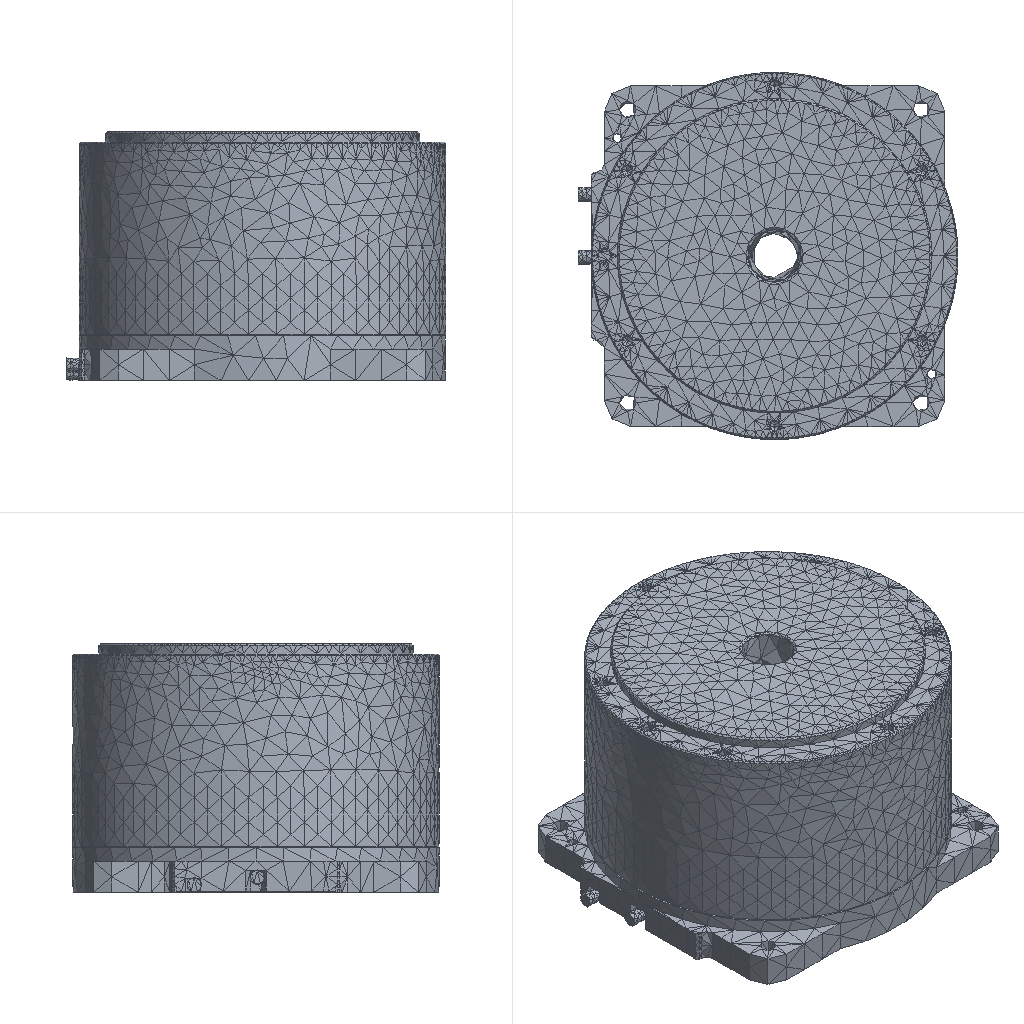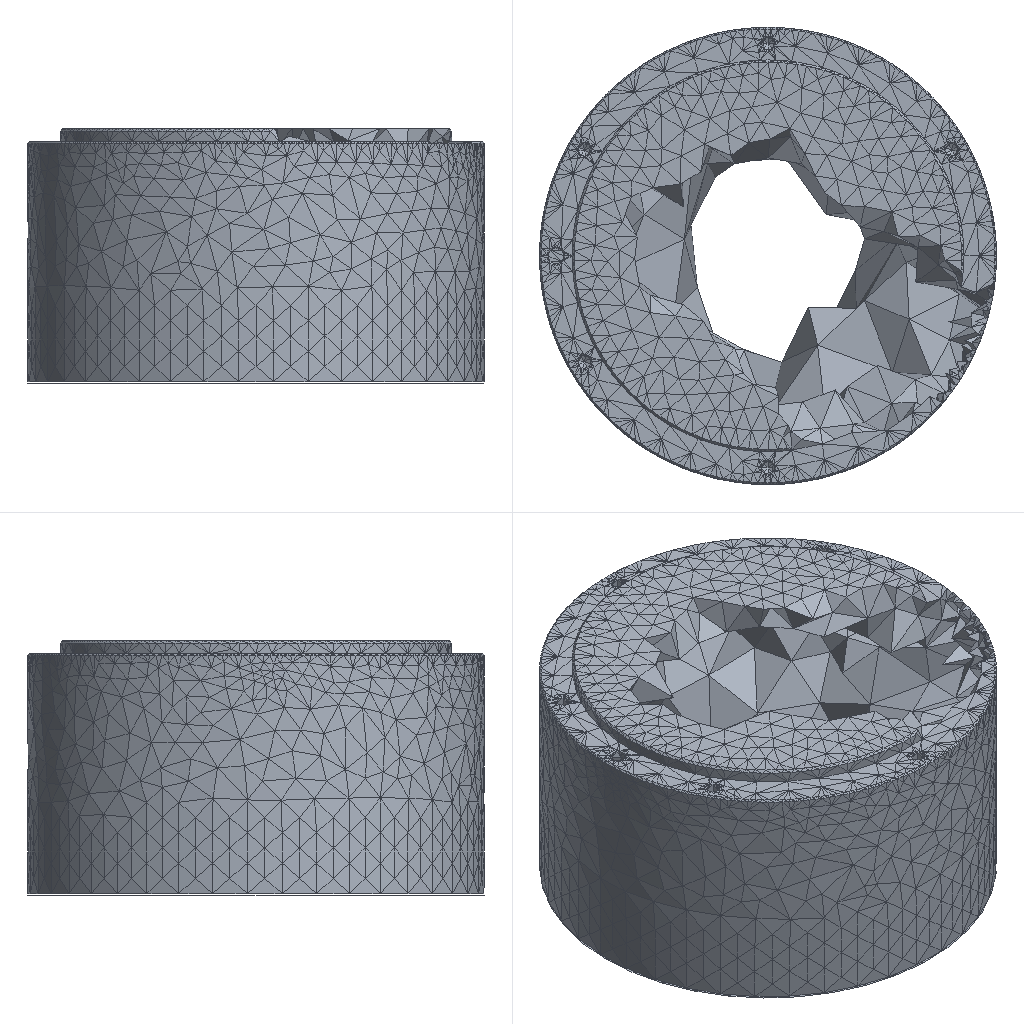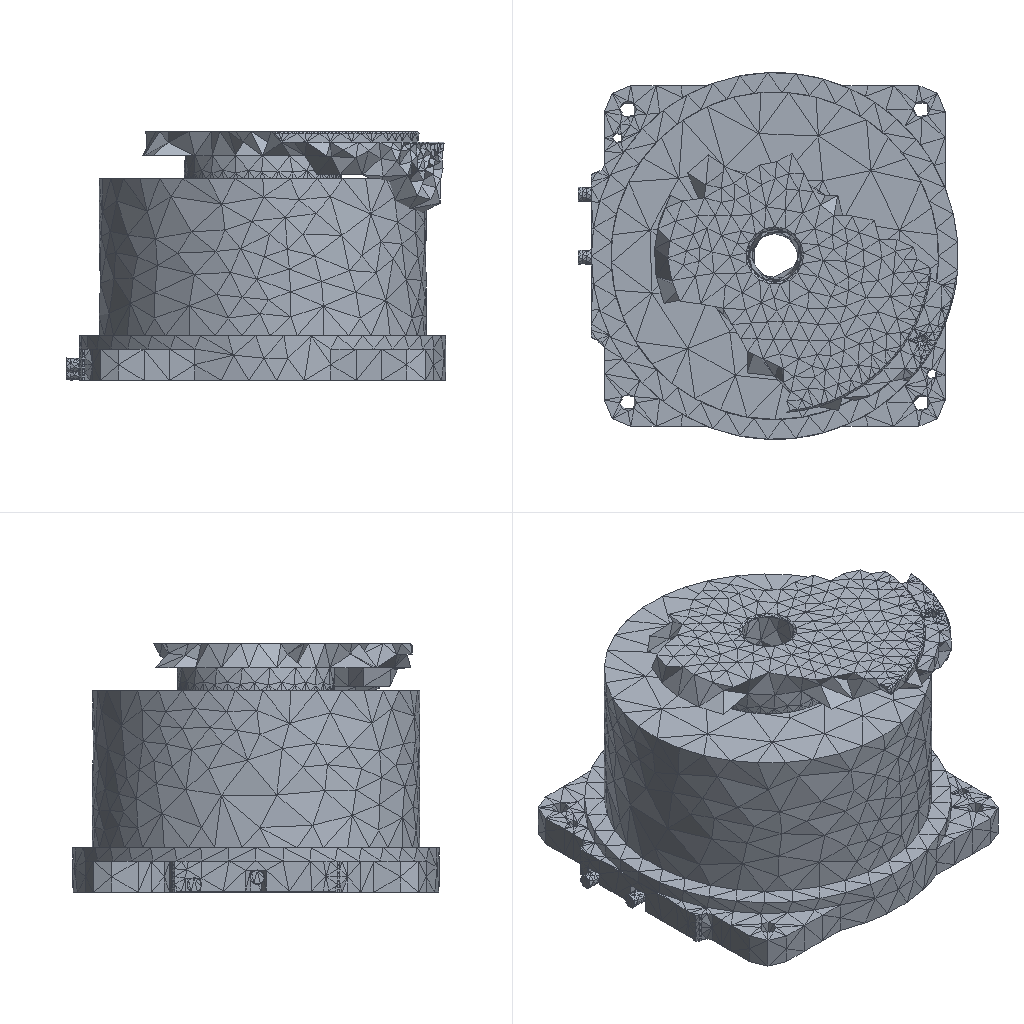Simulation study | ansys workbench
Set-up summary:
category,name,step,type,value,unit,region
solver,ansys_workbench
units,mm-N-s-tonne (MPa),,stated,"/units,MPA"
analysis,deck-1/LS1,,static
load_step,deck-1/LS1,deck-1/LS1,static,nsubst=1; time=1
analysis,deck-2/LS1,,modal,restart=True; perturbation=True; method=lanb; n_modes=6
load_step,deck-2/LS1,deck-2/LS1,modal
load_step,deck-2/LS1,deck-2/LS1,modal
mesh,deck-1.dat,,nodes,36561
mesh,deck-1.dat,,elements,23047
element_type,SOLID187,,,20568,,deck-1.dat
element_type,CONTA174,,,2058,,deck-1.dat
element_type,TARGE170,,,421,,deck-1.dat
mesh,deck-2.dat,,nodes,0
mesh,deck-2.dat,,elements,0
mesh,deck-2.dat,,note,"restart analysis: no node block, runs on the mesh of the upstream system's deck"
material,Structural Steel,,E,200000,tonne s^-2 mm^-1
material,Structural Steel,,nu,0.3
material,Structural Steel,,density,7.85e-09,tonne mm^-3
material,Structural Steel,,conductivity,60.5,tonne mm s^-3 C^-1
material,Structural Steel,,specific_heat,4.34e+08,mm^2 s^-2 C^-1
material,Structural Steel,,cte,1.2e-05,C^-1
material,Structural Steel,,permeability,10000
material,Structural Steel,,resistivity,0.00017,ohm mm
load,,deck-1/LS1,moment,"5000 [dir=(0, 0, 1) n=3]",,all
bc,Fixed Supports,deck-1/model,fixed,[dofs=ALL],,_FIXEDSU
contact,Contact Region,,bonded (always),element=CONTA174
contact,Contact Region 2,,bonded (always),element=CONTA174
contact,Contact Region 3,,bonded (always),element=CONTA174
contact,contact 4,,bonded (always),element=CONTA174
named_set,_CM49_FIXEDSU,,node,650
named_set,_FIXEDSU,,node,650
Results summary:
result,analyses[0].index,,,1
result,analyses[0].system,,,SYS
result,analyses[0].deck,,,deck-1.dat
result,analyses[0].solve_status,,,completed
result,analyses[0].analysis_type,,,static
result,analyses[0].physics,,,mechanical
result,analyses[0].unit_system,,,"NMM: mm, ton, N, s, mV, mA, degC"
result,analyses[0].n_sets,,,1
result,analyses[0].load_steps[0].set,set=1,,1
result,analyses[0].load_steps[0].time_or_freq,set=1,,1
result,analyses[0].load_steps[0].max_displacement_magnitude,set=1,,9.84173e-06
result,analyses[0].load_steps[0].max_von_mises_nodal,set=1,,0.2004
result,analyses[0].load_steps[0].reaction_force_sum_xyz[1],set=1,,-6.78179e-08
result,analyses[0].load_steps[0].reaction_force_sum_xyz[2],set=1,,-6.04514e-08
result,analyses[0].load_steps[0].reaction_force_sum_xyz[3],set=1,,6.76563e-08
result,analyses[1].index,,,2
result,analyses[1].system,,,SYS-1
result,analyses[1].deck,,,deck-2.dat
result,analyses[1].solve_status,,,completed
result,analyses[1].analysis_type,,,modal
result,analyses[1].physics,,,mechanical
result,analyses[1].unit_system,,,"NMM: mm, ton, N, s, mV, mA, degC"
result,analyses[1].n_sets,,,6
result,analyses[1].modal_frequencies_hz[1],,,4475.3
result,analyses[1].modal_frequencies_hz[2],,,4770.8
result,analyses[1].modal_frequencies_hz[3],,,6640.65
result,analyses[1].modal_frequencies_hz[4],,,7091.97
result,analyses[1].modal_frequencies_hz[5],,,8059.61
result,analyses[1].modal_frequencies_hz[6],,,8197.4